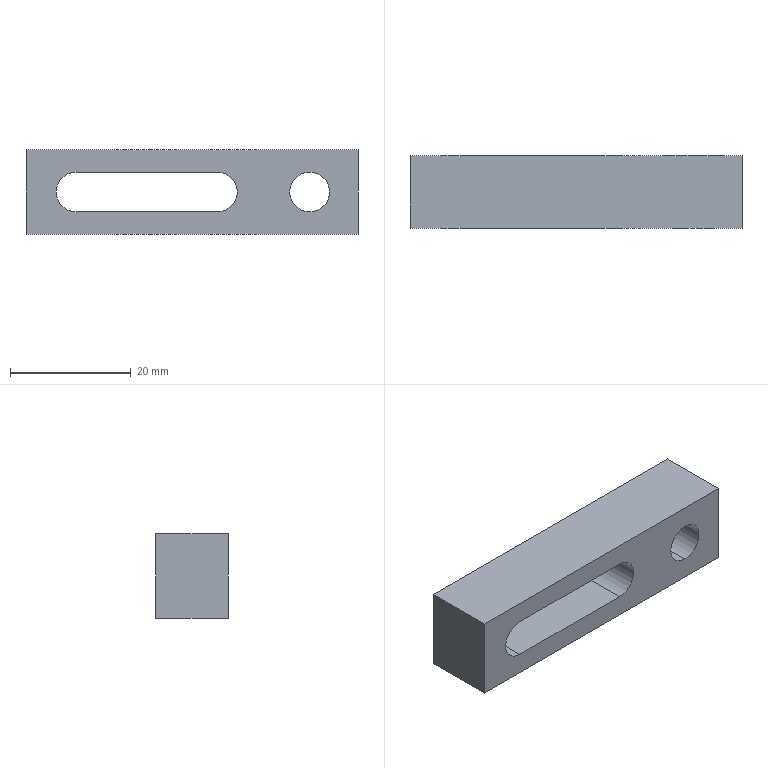Part | NX | features BREP 1 | 1 solid | 15 faces | box 55 x 12 x 14 mm | volume 6152 mm3 | plane 9 | cylinder 6 | commonest cylinder face diameters 6.6 x4 11 x2
STEP:
#1=CARTESIAN_POINT('',(19.5,-0.8,-5.5));
#2=VERTEX_POINT('',#1);
#3=CARTESIAN_POINT('',(19.5,-0.8,5.5));
#4=VERTEX_POINT('',#3);
#5=CARTESIAN_POINT('',(19.5,-0.8,0.));
#6=DIRECTION('',(0.,1.,0.));
#7=DIRECTION('',(0.,0.,1.));
#8=AXIS2_PLACEMENT_3D('',#5,#6,#7);
#9=CIRCLE('',#8,5.5);
#10=EDGE_CURVE('',#2,#4,#9,.T.);
#11=ORIENTED_EDGE('',*,*,#10,.F.);
#12=CARTESIAN_POINT('',(19.5,6.,-5.5));
#13=VERTEX_POINT('',#12);
#14=CARTESIAN_POINT('',(19.5,6.,-5.5));
#15=DIRECTION('',(0.,1.,0.));
#16=VECTOR('',#15,1000.);
#17=LINE('',#14,#16);
#18=EDGE_CURVE('',#2,#13,#17,.T.);
#19=ORIENTED_EDGE('',*,*,#18,.T.);
#20=CARTESIAN_POINT('',(19.5,6.,5.5));
#21=VERTEX_POINT('',#20);
#22=CARTESIAN_POINT('',(19.5,6.,0.));
#23=DIRECTION('',(0.,1.,0.));
#24=DIRECTION('',(0.,0.,1.));
#25=AXIS2_PLACEMENT_3D('',#22,#23,#24);
#26=CIRCLE('',#25,5.5);
#27=EDGE_CURVE('',#13,#21,#26,.T.);
#28=ORIENTED_EDGE('',*,*,#27,.T.);
#29=CARTESIAN_POINT('',(19.5,6.,5.5));
#30=DIRECTION('',(0.,1.,0.));
#31=VECTOR('',#30,1000.);
#32=LINE('',#29,#31);
#33=EDGE_CURVE('',#4,#21,#32,.T.);
#34=ORIENTED_EDGE('',*,*,#33,.F.);
#35=EDGE_LOOP('',(#11,#19,#28,#34));
#36=FACE_BOUND('',#35,.T.);
#37=CARTESIAN_POINT('',(19.5,6.,0.));
#38=DIRECTION('',(0.,1.,0.));
#39=DIRECTION('',(0.,0.,-1.));
#40=AXIS2_PLACEMENT_3D('',#37,#38,#39);
#41=CYLINDRICAL_SURFACE('',#40,5.5);
#42=ADVANCED_FACE('',(#36),#41,.F.);
#43=CARTESIAN_POINT('',(19.5,-6.,-3.3));
#44=VERTEX_POINT('',#43);
#45=CARTESIAN_POINT('',(19.5,-6.,3.3));
#46=VERTEX_POINT('',#45);
#47=CARTESIAN_POINT('',(19.5,-6.,0.));
#48=DIRECTION('',(0.,1.,0.));
#49=DIRECTION('',(0.,0.,1.));
#50=AXIS2_PLACEMENT_3D('',#47,#48,#49);
#51=CIRCLE('',#50,3.3);
#52=EDGE_CURVE('',#44,#46,#51,.T.);
#53=ORIENTED_EDGE('',*,*,#52,.F.);
#54=CARTESIAN_POINT('',(19.5,-0.8,-3.3));
#55=VERTEX_POINT('',#54);
#56=CARTESIAN_POINT('',(19.5,6.,-3.3));
#57=DIRECTION('',(0.,1.,0.));
#58=VECTOR('',#57,1000.);
#59=LINE('',#56,#58);
#60=EDGE_CURVE('',#44,#55,#59,.T.);
#61=ORIENTED_EDGE('',*,*,#60,.T.);
#62=CARTESIAN_POINT('',(19.5,-0.8,3.3));
#63=VERTEX_POINT('',#62);
#64=CARTESIAN_POINT('',(19.5,-0.8,0.));
#65=DIRECTION('',(0.,1.,0.));
#66=DIRECTION('',(0.,0.,1.));
#67=AXIS2_PLACEMENT_3D('',#64,#65,#66);
#68=CIRCLE('',#67,3.3);
#69=EDGE_CURVE('',#55,#63,#68,.T.);
#70=ORIENTED_EDGE('',*,*,#69,.T.);
#71=CARTESIAN_POINT('',(19.5,6.,3.3));
#72=DIRECTION('',(0.,1.,0.));
#73=VECTOR('',#72,1000.);
#74=LINE('',#71,#73);
#75=EDGE_CURVE('',#46,#63,#74,.T.);
#76=ORIENTED_EDGE('',*,*,#75,.F.);
#77=EDGE_LOOP('',(#53,#61,#70,#76));
#78=FACE_BOUND('',#77,.T.);
#79=CARTESIAN_POINT('',(19.5,6.,0.));
#80=DIRECTION('',(0.,1.,0.));
#81=DIRECTION('',(0.,0.,-1.));
#82=AXIS2_PLACEMENT_3D('',#79,#80,#81);
#83=CYLINDRICAL_SURFACE('',#82,3.3);
#84=ADVANCED_FACE('',(#78),#83,.F.);
#85=CARTESIAN_POINT('',(27.5,-6.,7.));
#86=VERTEX_POINT('',#85);
#87=CARTESIAN_POINT('',(27.5,-6.,-7.));
#88=VERTEX_POINT('',#87);
#89=CARTESIAN_POINT('',(27.5,-6.,-7.));
#90=DIRECTION('',(0.,0.,-1.));
#91=VECTOR('',#90,1000.);
#92=LINE('',#89,#91);
#93=EDGE_CURVE('',#86,#88,#92,.T.);
#94=ORIENTED_EDGE('',*,*,#93,.T.);
#95=CARTESIAN_POINT('',(27.5,6.,-7.));
#96=VERTEX_POINT('',#95);
#97=CARTESIAN_POINT('',(27.5,6.,-7.));
#98=DIRECTION('',(0.,-1.,0.));
#99=VECTOR('',#98,1000.);
#100=LINE('',#97,#99);
#101=EDGE_CURVE('',#96,#88,#100,.T.);
#102=ORIENTED_EDGE('',*,*,#101,.F.);
#103=CARTESIAN_POINT('',(27.5,6.,7.));
#104=VERTEX_POINT('',#103);
#105=CARTESIAN_POINT('',(27.5,6.,-7.));
#106=DIRECTION('',(0.,0.,-1.));
#107=VECTOR('',#106,1000.);
#108=LINE('',#105,#107);
#109=EDGE_CURVE('',#104,#96,#108,.T.);
#110=ORIENTED_EDGE('',*,*,#109,.F.);
#111=CARTESIAN_POINT('',(27.5,6.,7.));
#112=DIRECTION('',(0.,-1.,0.));
#113=VECTOR('',#112,1000.);
#114=LINE('',#111,#113);
#115=EDGE_CURVE('',#104,#86,#114,.T.);
#116=ORIENTED_EDGE('',*,*,#115,.T.);
#117=EDGE_LOOP('',(#94,#102,#110,#116));
#118=FACE_BOUND('',#117,.T.);
#119=CARTESIAN_POINT('',(27.5,6.,-7.));
#120=DIRECTION('',(-1.,0.,0.));
#121=DIRECTION('',(0.,0.,-1.));
#122=AXIS2_PLACEMENT_3D('',#119,#120,#121);
#123=PLANE('',#122);
#124=ADVANCED_FACE('',(#118),#123,.F.);
#125=CARTESIAN_POINT('',(-27.5,-6.,-7.));
#126=VERTEX_POINT('',#125);
#127=CARTESIAN_POINT('',(-27.5,-6.,-7.));
#128=DIRECTION('',(-1.,0.,0.));
#129=VECTOR('',#128,1000.);
#130=LINE('',#127,#129);
#131=EDGE_CURVE('',#88,#126,#130,.T.);
#132=ORIENTED_EDGE('',*,*,#131,.T.);
#133=CARTESIAN_POINT('',(-27.5,6.,-7.));
#134=VERTEX_POINT('',#133);
#135=CARTESIAN_POINT('',(-27.5,6.,-7.));
#136=DIRECTION('',(0.,-1.,0.));
#137=VECTOR('',#136,1000.);
#138=LINE('',#135,#137);
#139=EDGE_CURVE('',#134,#126,#138,.T.);
#140=ORIENTED_EDGE('',*,*,#139,.F.);
#141=CARTESIAN_POINT('',(-27.5,6.,-7.));
#142=DIRECTION('',(-1.,0.,0.));
#143=VECTOR('',#142,1000.);
#144=LINE('',#141,#143);
#145=EDGE_CURVE('',#96,#134,#144,.T.);
#146=ORIENTED_EDGE('',*,*,#145,.F.);
#147=ORIENTED_EDGE('',*,*,#101,.T.);
#148=EDGE_LOOP('',(#132,#140,#146,#147));
#149=FACE_BOUND('',#148,.T.);
#150=CARTESIAN_POINT('',(-27.5,6.,-7.));
#151=DIRECTION('',(0.,0.,1.));
#152=DIRECTION('',(-1.,0.,0.));
#153=AXIS2_PLACEMENT_3D('',#150,#151,#152);
#154=PLANE('',#153);
#155=ADVANCED_FACE('',(#149),#154,.F.);
#156=CARTESIAN_POINT('',(-27.5,-6.,7.));
#157=VERTEX_POINT('',#156);
#158=CARTESIAN_POINT('',(-27.5,-6.,-7.));
#159=DIRECTION('',(0.,0.,1.));
#160=VECTOR('',#159,1000.);
#161=LINE('',#158,#160);
#162=EDGE_CURVE('',#126,#157,#161,.T.);
#163=ORIENTED_EDGE('',*,*,#162,.T.);
#164=CARTESIAN_POINT('',(-27.5,6.,7.));
#165=VERTEX_POINT('',#164);
#166=CARTESIAN_POINT('',(-27.5,6.,7.));
#167=DIRECTION('',(0.,-1.,0.));
#168=VECTOR('',#167,1000.);
#169=LINE('',#166,#168);
#170=EDGE_CURVE('',#165,#157,#169,.T.);
#171=ORIENTED_EDGE('',*,*,#170,.F.);
#172=CARTESIAN_POINT('',(-27.5,6.,-7.));
#173=DIRECTION('',(0.,0.,1.));
#174=VECTOR('',#173,1000.);
#175=LINE('',#172,#174);
#176=EDGE_CURVE('',#134,#165,#175,.T.);
#177=ORIENTED_EDGE('',*,*,#176,.F.);
#178=ORIENTED_EDGE('',*,*,#139,.T.);
#179=EDGE_LOOP('',(#163,#171,#177,#178));
#180=FACE_BOUND('',#179,.T.);
#181=CARTESIAN_POINT('',(-27.5,6.,-7.));
#182=DIRECTION('',(1.,0.,0.));
#183=DIRECTION('',(0.,0.,1.));
#184=AXIS2_PLACEMENT_3D('',#181,#182,#183);
#185=PLANE('',#184);
#186=ADVANCED_FACE('',(#180),#185,.F.);
#187=CARTESIAN_POINT('',(-27.5,-6.,7.));
#188=DIRECTION('',(1.,0.,0.));
#189=VECTOR('',#188,1000.);
#190=LINE('',#187,#189);
#191=EDGE_CURVE('',#157,#86,#190,.T.);
#192=ORIENTED_EDGE('',*,*,#191,.T.);
#193=ORIENTED_EDGE('',*,*,#115,.F.);
#194=CARTESIAN_POINT('',(-27.5,6.,7.));
#195=DIRECTION('',(1.,0.,0.));
#196=VECTOR('',#195,1000.);
#197=LINE('',#194,#196);
#198=EDGE_CURVE('',#165,#104,#197,.T.);
#199=ORIENTED_EDGE('',*,*,#198,.F.);
#200=ORIENTED_EDGE('',*,*,#170,.T.);
#201=EDGE_LOOP('',(#192,#193,#199,#200));
#202=FACE_BOUND('',#201,.T.);
#203=CARTESIAN_POINT('',(-27.5,6.,7.));
#204=DIRECTION('',(0.,0.,-1.));
#205=DIRECTION('',(1.,0.,0.));
#206=AXIS2_PLACEMENT_3D('',#203,#204,#205);
#207=PLANE('',#206);
#208=ADVANCED_FACE('',(#202),#207,.F.);
#209=CARTESIAN_POINT('',(4.2,6.,3.3));
#210=VERTEX_POINT('',#209);
#211=CARTESIAN_POINT('',(4.2,6.,-3.3));
#212=VERTEX_POINT('',#211);
#213=CARTESIAN_POINT('',(4.2,6.,0.));
#214=DIRECTION('',(0.,1.,0.));
#215=DIRECTION('',(0.,0.,1.));
#216=AXIS2_PLACEMENT_3D('',#213,#214,#215);
#217=CIRCLE('',#216,3.3);
#218=EDGE_CURVE('',#210,#212,#217,.T.);
#219=ORIENTED_EDGE('',*,*,#218,.F.);
#220=CARTESIAN_POINT('',(-19.2,6.,3.3));
#221=VERTEX_POINT('',#220);
#222=CARTESIAN_POINT('',(-19.2,6.,3.3));
#223=DIRECTION('',(1.,0.,0.));
#224=VECTOR('',#223,1000.);
#225=LINE('',#222,#224);
#226=EDGE_CURVE('',#221,#210,#225,.T.);
#227=ORIENTED_EDGE('',*,*,#226,.F.);
#228=CARTESIAN_POINT('',(-19.2,6.,-3.3));
#229=VERTEX_POINT('',#228);
#230=CARTESIAN_POINT('',(-19.2,6.,0.));
#231=DIRECTION('',(0.,1.,0.));
#232=DIRECTION('',(0.,0.,1.));
#233=AXIS2_PLACEMENT_3D('',#230,#231,#232);
#234=CIRCLE('',#233,3.3);
#235=EDGE_CURVE('',#229,#221,#234,.T.);
#236=ORIENTED_EDGE('',*,*,#235,.F.);
#237=CARTESIAN_POINT('',(-19.2,6.,-3.3));
#238=DIRECTION('',(1.,0.,0.));
#239=VECTOR('',#238,1000.);
#240=LINE('',#237,#239);
#241=EDGE_CURVE('',#229,#212,#240,.T.);
#242=ORIENTED_EDGE('',*,*,#241,.T.);
#243=EDGE_LOOP('',(#219,#227,#236,#242));
#244=FACE_BOUND('',#243,.T.);
#245=CARTESIAN_POINT('',(19.5,6.,0.));
#246=DIRECTION('',(0.,1.,0.));
#247=DIRECTION('',(0.,0.,1.));
#248=AXIS2_PLACEMENT_3D('',#245,#246,#247);
#249=CIRCLE('',#248,5.5);
#250=EDGE_CURVE('',#21,#13,#249,.T.);
#251=ORIENTED_EDGE('',*,*,#250,.F.);
#252=ORIENTED_EDGE('',*,*,#27,.F.);
#253=EDGE_LOOP('',(#251,#252));
#254=FACE_BOUND('',#253,.T.);
#255=ORIENTED_EDGE('',*,*,#109,.T.);
#256=ORIENTED_EDGE('',*,*,#145,.T.);
#257=ORIENTED_EDGE('',*,*,#176,.T.);
#258=ORIENTED_EDGE('',*,*,#198,.T.);
#259=EDGE_LOOP('',(#255,#256,#257,#258));
#260=FACE_BOUND('',#259,.T.);
#261=CARTESIAN_POINT('',(0.,6.,0.));
#262=DIRECTION('',(0.,1.,0.));
#263=DIRECTION('',(0.,0.,-1.));
#264=AXIS2_PLACEMENT_3D('',#261,#262,#263);
#265=PLANE('',#264);
#266=ADVANCED_FACE('',(#244,#254,#260),#265,.T.);
#267=CARTESIAN_POINT('',(-19.2,-6.,-3.3));
#268=VERTEX_POINT('',#267);
#269=CARTESIAN_POINT('',(4.2,-6.,-3.3));
#270=VERTEX_POINT('',#269);
#271=CARTESIAN_POINT('',(-19.2,-6.,-3.3));
#272=DIRECTION('',(1.,0.,0.));
#273=VECTOR('',#272,1000.);
#274=LINE('',#271,#273);
#275=EDGE_CURVE('',#268,#270,#274,.T.);
#276=ORIENTED_EDGE('',*,*,#275,.F.);
#277=CARTESIAN_POINT('',(-19.2,-6.,3.3));
#278=VERTEX_POINT('',#277);
#279=CARTESIAN_POINT('',(-19.2,-6.,0.));
#280=DIRECTION('',(0.,1.,0.));
#281=DIRECTION('',(0.,0.,1.));
#282=AXIS2_PLACEMENT_3D('',#279,#280,#281);
#283=CIRCLE('',#282,3.3);
#284=EDGE_CURVE('',#268,#278,#283,.T.);
#285=ORIENTED_EDGE('',*,*,#284,.T.);
#286=CARTESIAN_POINT('',(4.2,-6.,3.3));
#287=VERTEX_POINT('',#286);
#288=CARTESIAN_POINT('',(-19.2,-6.,3.3));
#289=DIRECTION('',(1.,0.,0.));
#290=VECTOR('',#289,1000.);
#291=LINE('',#288,#290);
#292=EDGE_CURVE('',#278,#287,#291,.T.);
#293=ORIENTED_EDGE('',*,*,#292,.T.);
#294=CARTESIAN_POINT('',(4.2,-6.,0.));
#295=DIRECTION('',(0.,1.,0.));
#296=DIRECTION('',(0.,0.,1.));
#297=AXIS2_PLACEMENT_3D('',#294,#295,#296);
#298=CIRCLE('',#297,3.3);
#299=EDGE_CURVE('',#287,#270,#298,.T.);
#300=ORIENTED_EDGE('',*,*,#299,.T.);
#301=EDGE_LOOP('',(#276,#285,#293,#300));
#302=FACE_BOUND('',#301,.T.);
#303=CARTESIAN_POINT('',(19.5,-6.,0.));
#304=DIRECTION('',(0.,1.,0.));
#305=DIRECTION('',(0.,0.,1.));
#306=AXIS2_PLACEMENT_3D('',#303,#304,#305);
#307=CIRCLE('',#306,3.3);
#308=EDGE_CURVE('',#46,#44,#307,.T.);
#309=ORIENTED_EDGE('',*,*,#308,.T.);
#310=ORIENTED_EDGE('',*,*,#52,.T.);
#311=EDGE_LOOP('',(#309,#310));
#312=FACE_BOUND('',#311,.T.);
#313=ORIENTED_EDGE('',*,*,#93,.F.);
#314=ORIENTED_EDGE('',*,*,#191,.F.);
#315=ORIENTED_EDGE('',*,*,#162,.F.);
#316=ORIENTED_EDGE('',*,*,#131,.F.);
#317=EDGE_LOOP('',(#313,#314,#315,#316));
#318=FACE_BOUND('',#317,.T.);
#319=CARTESIAN_POINT('',(0.,-6.,0.));
#320=DIRECTION('',(0.,1.,0.));
#321=DIRECTION('',(0.,0.,-1.));
#322=AXIS2_PLACEMENT_3D('',#319,#320,#321);
#323=PLANE('',#322);
#324=ADVANCED_FACE('',(#302,#312,#318),#323,.F.);
#325=ORIENTED_EDGE('',*,*,#60,.F.);
#326=ORIENTED_EDGE('',*,*,#308,.F.);
#327=ORIENTED_EDGE('',*,*,#75,.T.);
#328=CARTESIAN_POINT('',(19.5,-0.8,0.));
#329=DIRECTION('',(0.,1.,0.));
#330=DIRECTION('',(0.,0.,1.));
#331=AXIS2_PLACEMENT_3D('',#328,#329,#330);
#332=CIRCLE('',#331,3.3);
#333=EDGE_CURVE('',#63,#55,#332,.T.);
#334=ORIENTED_EDGE('',*,*,#333,.T.);
#335=EDGE_LOOP('',(#325,#326,#327,#334));
#336=FACE_BOUND('',#335,.T.);
#337=CARTESIAN_POINT('',(19.5,6.,0.));
#338=DIRECTION('',(0.,1.,0.));
#339=DIRECTION('',(0.,0.,-1.));
#340=AXIS2_PLACEMENT_3D('',#337,#338,#339);
#341=CYLINDRICAL_SURFACE('',#340,3.3);
#342=ADVANCED_FACE('',(#336),#341,.F.);
#343=ORIENTED_EDGE('',*,*,#333,.F.);
#344=ORIENTED_EDGE('',*,*,#69,.F.);
#345=EDGE_LOOP('',(#343,#344));
#346=FACE_BOUND('',#345,.T.);
#347=CARTESIAN_POINT('',(19.5,-0.8,0.));
#348=DIRECTION('',(0.,1.,0.));
#349=DIRECTION('',(0.,0.,1.));
#350=AXIS2_PLACEMENT_3D('',#347,#348,#349);
#351=CIRCLE('',#350,5.5);
#352=EDGE_CURVE('',#4,#2,#351,.T.);
#353=ORIENTED_EDGE('',*,*,#352,.T.);
#354=ORIENTED_EDGE('',*,*,#10,.T.);
#355=EDGE_LOOP('',(#353,#354));
#356=FACE_BOUND('',#355,.T.);
#357=CARTESIAN_POINT('',(22.8,-0.8,0.));
#358=DIRECTION('',(0.,-1.,0.));
#359=DIRECTION('',(0.,0.,1.));
#360=AXIS2_PLACEMENT_3D('',#357,#358,#359);
#361=PLANE('',#360);
#362=ADVANCED_FACE('',(#346,#356),#361,.F.);
#363=ORIENTED_EDGE('',*,*,#18,.F.);
#364=ORIENTED_EDGE('',*,*,#352,.F.);
#365=ORIENTED_EDGE('',*,*,#33,.T.);
#366=ORIENTED_EDGE('',*,*,#250,.T.);
#367=EDGE_LOOP('',(#363,#364,#365,#366));
#368=FACE_BOUND('',#367,.T.);
#369=CARTESIAN_POINT('',(19.5,6.,0.));
#370=DIRECTION('',(0.,1.,0.));
#371=DIRECTION('',(0.,0.,-1.));
#372=AXIS2_PLACEMENT_3D('',#369,#370,#371);
#373=CYLINDRICAL_SURFACE('',#372,5.5);
#374=ADVANCED_FACE('',(#368),#373,.F.);
#375=ORIENTED_EDGE('',*,*,#299,.F.);
#376=CARTESIAN_POINT('',(4.2,6.,3.3));
#377=DIRECTION('',(0.,-1.,0.));
#378=VECTOR('',#377,1000.);
#379=LINE('',#376,#378);
#380=EDGE_CURVE('',#210,#287,#379,.T.);
#381=ORIENTED_EDGE('',*,*,#380,.F.);
#382=ORIENTED_EDGE('',*,*,#218,.T.);
#383=CARTESIAN_POINT('',(4.2,6.,-3.3));
#384=DIRECTION('',(0.,1.,0.));
#385=VECTOR('',#384,1000.);
#386=LINE('',#383,#385);
#387=EDGE_CURVE('',#270,#212,#386,.T.);
#388=ORIENTED_EDGE('',*,*,#387,.F.);
#389=EDGE_LOOP('',(#375,#381,#382,#388));
#390=FACE_BOUND('',#389,.T.);
#391=CARTESIAN_POINT('',(4.2,6.,0.));
#392=DIRECTION('',(0.,1.,0.));
#393=DIRECTION('',(0.,0.,-1.));
#394=AXIS2_PLACEMENT_3D('',#391,#392,#393);
#395=CYLINDRICAL_SURFACE('',#394,3.3);
#396=ADVANCED_FACE('',(#390),#395,.F.);
#397=ORIENTED_EDGE('',*,*,#235,.T.);
#398=CARTESIAN_POINT('',(-19.2,6.,3.3));
#399=DIRECTION('',(0.,1.,0.));
#400=VECTOR('',#399,1000.);
#401=LINE('',#398,#400);
#402=EDGE_CURVE('',#278,#221,#401,.T.);
#403=ORIENTED_EDGE('',*,*,#402,.F.);
#404=ORIENTED_EDGE('',*,*,#284,.F.);
#405=CARTESIAN_POINT('',(-19.2,6.,-3.3));
#406=DIRECTION('',(0.,-1.,0.));
#407=VECTOR('',#406,1000.);
#408=LINE('',#405,#407);
#409=EDGE_CURVE('',#229,#268,#408,.T.);
#410=ORIENTED_EDGE('',*,*,#409,.F.);
#411=EDGE_LOOP('',(#397,#403,#404,#410));
#412=FACE_BOUND('',#411,.T.);
#413=CARTESIAN_POINT('',(-19.2,6.,0.));
#414=DIRECTION('',(0.,1.,0.));
#415=DIRECTION('',(0.,0.,-1.));
#416=AXIS2_PLACEMENT_3D('',#413,#414,#415);
#417=CYLINDRICAL_SURFACE('',#416,3.3);
#418=ADVANCED_FACE('',(#412),#417,.F.);
#419=ORIENTED_EDGE('',*,*,#387,.T.);
#420=ORIENTED_EDGE('',*,*,#241,.F.);
#421=ORIENTED_EDGE('',*,*,#409,.T.);
#422=ORIENTED_EDGE('',*,*,#275,.T.);
#423=EDGE_LOOP('',(#419,#420,#421,#422));
#424=FACE_BOUND('',#423,.T.);
#425=CARTESIAN_POINT('',(-19.2,6.,-3.3));
#426=DIRECTION('',(0.,0.,-1.));
#427=DIRECTION('',(1.,0.,0.));
#428=AXIS2_PLACEMENT_3D('',#425,#426,#427);
#429=PLANE('',#428);
#430=ADVANCED_FACE('',(#424),#429,.F.);
#431=ORIENTED_EDGE('',*,*,#380,.T.);
#432=ORIENTED_EDGE('',*,*,#292,.F.);
#433=ORIENTED_EDGE('',*,*,#402,.T.);
#434=ORIENTED_EDGE('',*,*,#226,.T.);
#435=EDGE_LOOP('',(#431,#432,#433,#434));
#436=FACE_BOUND('',#435,.T.);
#437=CARTESIAN_POINT('',(-19.2,6.,3.3));
#438=DIRECTION('',(0.,0.,1.));
#439=DIRECTION('',(-1.,0.,0.));
#440=AXIS2_PLACEMENT_3D('',#437,#438,#439);
#441=PLANE('',#440);
#442=ADVANCED_FACE('',(#436),#441,.F.);
#443=CLOSED_SHELL('',(#42,#84,#124,#155,#186,#208,#266,#324,#342,#362,#374,#396,#418,#430,#442));
#444=MANIFOLD_SOLID_BREP('',#443);
#445=(LENGTH_UNIT()NAMED_UNIT(*)SI_UNIT(.MILLI.,.METRE.));
#446=UNCERTAINTY_MEASURE_WITH_UNIT(LENGTH_MEASURE(0.00001),#445,'','');
#447=(NAMED_UNIT(*)PLANE_ANGLE_UNIT()SI_UNIT($,.RADIAN.));
#448=(NAMED_UNIT(*)SI_UNIT($,.STERADIAN.)SOLID_ANGLE_UNIT());
#449=(GEOMETRIC_REPRESENTATION_CONTEXT(3)GLOBAL_UNCERTAINTY_ASSIGNED_CONTEXT((#446))GLOBAL_UNIT_ASSIGNED_CONTEXT((#445,#447,#448))REPRESENTATION_CONTEXT('',''));
#450=ADVANCED_BREP_SHAPE_REPRESENTATION('',(#444),#449);